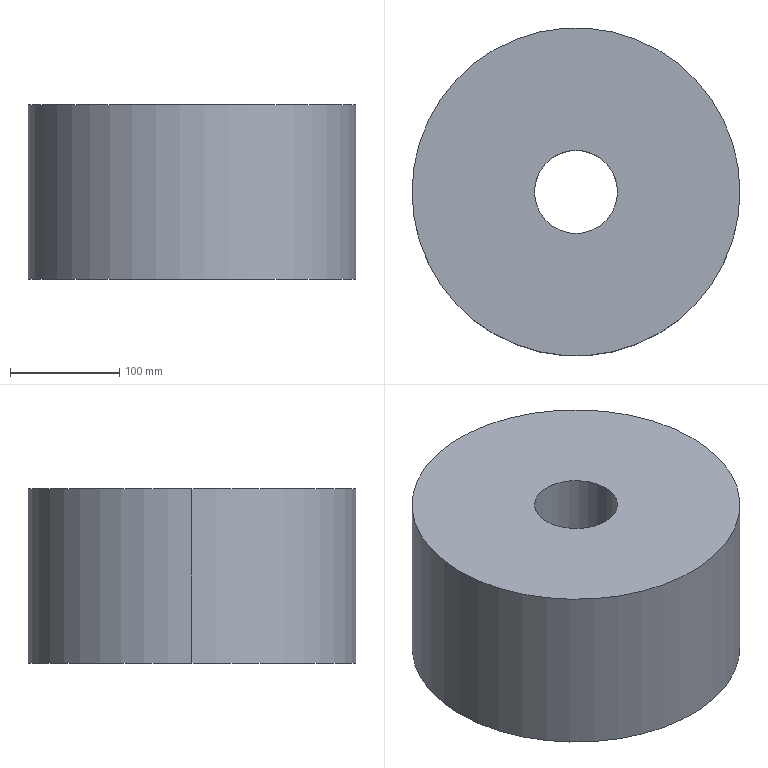Part | SolidWorks | features Extrusion 1 | 1 solid | 6 faces | box 300 x 300 x 160 mm | volume 10583900 mm3 | cylinder 4 | plane 2 | commonest cylinder face diameters 76 x2 300 x2
STEP:
#1=CARTESIAN_POINT('',(-38.,0.,80.));
#2=VERTEX_POINT('',#1);
#3=CARTESIAN_POINT('',(38.,0.,80.));
#4=VERTEX_POINT('',#3);
#5=CARTESIAN_POINT('',(0.,0.,80.));
#6=DIRECTION('',(0.,0.,1.));
#7=DIRECTION('',(1.,0.,0.));
#8=AXIS2_PLACEMENT_3D('',#5,#6,#7);
#9=CIRCLE('',#8,38.);
#10=EDGE_CURVE('',#2,#4,#9,.T.);
#11=ORIENTED_EDGE('',*,*,#10,.T.);
#12=CARTESIAN_POINT('',(38.,0.,-80.));
#13=VERTEX_POINT('',#12);
#14=CARTESIAN_POINT('',(38.,0.,80.));
#15=DIRECTION('',(0.,0.,-1.));
#16=VECTOR('',#15,1000.);
#17=LINE('',#14,#16);
#18=EDGE_CURVE('',#4,#13,#17,.T.);
#19=ORIENTED_EDGE('',*,*,#18,.T.);
#20=CARTESIAN_POINT('',(-38.,0.,-80.));
#21=VERTEX_POINT('',#20);
#22=CARTESIAN_POINT('',(0.,0.,-80.));
#23=DIRECTION('',(0.,0.,1.));
#24=DIRECTION('',(1.,0.,0.));
#25=AXIS2_PLACEMENT_3D('',#22,#23,#24);
#26=CIRCLE('',#25,38.);
#27=EDGE_CURVE('',#21,#13,#26,.T.);
#28=ORIENTED_EDGE('',*,*,#27,.F.);
#29=CARTESIAN_POINT('',(-38.,0.,80.));
#30=DIRECTION('',(0.,0.,-1.));
#31=VECTOR('',#30,1000.);
#32=LINE('',#29,#31);
#33=EDGE_CURVE('',#2,#21,#32,.T.);
#34=ORIENTED_EDGE('',*,*,#33,.F.);
#35=EDGE_LOOP('',(#11,#19,#28,#34));
#36=FACE_OUTER_BOUND('',#35,.T.);
#37=CARTESIAN_POINT('',(0.,0.,80.));
#38=DIRECTION('',(0.,0.,-1.));
#39=DIRECTION('',(-1.,0.,0.));
#40=AXIS2_PLACEMENT_3D('',#37,#38,#39);
#41=CYLINDRICAL_SURFACE('',#40,38.);
#42=ADVANCED_FACE('',(#36),#41,.F.);
#43=CARTESIAN_POINT('',(150.,0.,80.));
#44=VERTEX_POINT('',#43);
#45=CARTESIAN_POINT('',(-150.,0.,80.));
#46=VERTEX_POINT('',#45);
#47=CARTESIAN_POINT('',(0.,0.,80.));
#48=DIRECTION('',(0.,0.,1.));
#49=DIRECTION('',(1.,0.,0.));
#50=AXIS2_PLACEMENT_3D('',#47,#48,#49);
#51=CIRCLE('',#50,150.);
#52=EDGE_CURVE('',#44,#46,#51,.T.);
#53=ORIENTED_EDGE('',*,*,#52,.F.);
#54=CARTESIAN_POINT('',(150.,0.,-80.));
#55=VERTEX_POINT('',#54);
#56=CARTESIAN_POINT('',(150.,0.,80.));
#57=DIRECTION('',(0.,0.,-1.));
#58=VECTOR('',#57,1000.);
#59=LINE('',#56,#58);
#60=EDGE_CURVE('',#44,#55,#59,.T.);
#61=ORIENTED_EDGE('',*,*,#60,.T.);
#62=CARTESIAN_POINT('',(-150.,0.,-80.));
#63=VERTEX_POINT('',#62);
#64=CARTESIAN_POINT('',(0.,0.,-80.));
#65=DIRECTION('',(0.,0.,1.));
#66=DIRECTION('',(1.,0.,0.));
#67=AXIS2_PLACEMENT_3D('',#64,#65,#66);
#68=CIRCLE('',#67,150.);
#69=EDGE_CURVE('',#55,#63,#68,.T.);
#70=ORIENTED_EDGE('',*,*,#69,.T.);
#71=CARTESIAN_POINT('',(-150.,0.,80.));
#72=DIRECTION('',(0.,0.,-1.));
#73=VECTOR('',#72,1000.);
#74=LINE('',#71,#73);
#75=EDGE_CURVE('',#46,#63,#74,.T.);
#76=ORIENTED_EDGE('',*,*,#75,.F.);
#77=EDGE_LOOP('',(#53,#61,#70,#76));
#78=FACE_OUTER_BOUND('',#77,.T.);
#79=CARTESIAN_POINT('',(0.,0.,80.));
#80=DIRECTION('',(0.,0.,-1.));
#81=DIRECTION('',(-1.,0.,0.));
#82=AXIS2_PLACEMENT_3D('',#79,#80,#81);
#83=CYLINDRICAL_SURFACE('',#82,150.);
#84=ADVANCED_FACE('',(#78),#83,.T.);
#85=CARTESIAN_POINT('',(0.,0.,80.));
#86=DIRECTION('',(0.,0.,1.));
#87=DIRECTION('',(1.,0.,0.));
#88=AXIS2_PLACEMENT_3D('',#85,#86,#87);
#89=CIRCLE('',#88,150.);
#90=EDGE_CURVE('',#46,#44,#89,.T.);
#91=ORIENTED_EDGE('',*,*,#90,.T.);
#92=ORIENTED_EDGE('',*,*,#52,.T.);
#93=EDGE_LOOP('',(#91,#92));
#94=FACE_OUTER_BOUND('',#93,.T.);
#95=ORIENTED_EDGE('',*,*,#10,.F.);
#96=CARTESIAN_POINT('',(0.,0.,80.));
#97=DIRECTION('',(0.,0.,1.));
#98=DIRECTION('',(1.,0.,0.));
#99=AXIS2_PLACEMENT_3D('',#96,#97,#98);
#100=CIRCLE('',#99,38.);
#101=EDGE_CURVE('',#4,#2,#100,.T.);
#102=ORIENTED_EDGE('',*,*,#101,.F.);
#103=EDGE_LOOP('',(#95,#102));
#104=FACE_BOUND('',#103,.T.);
#105=CARTESIAN_POINT('',(0.,0.,80.));
#106=DIRECTION('',(0.,0.,1.));
#107=DIRECTION('',(1.,0.,0.));
#108=AXIS2_PLACEMENT_3D('',#105,#106,#107);
#109=PLANE('',#108);
#110=ADVANCED_FACE('',(#94,#104),#109,.T.);
#111=CARTESIAN_POINT('',(0.,0.,-80.));
#112=DIRECTION('',(0.,0.,1.));
#113=DIRECTION('',(1.,0.,0.));
#114=AXIS2_PLACEMENT_3D('',#111,#112,#113);
#115=CIRCLE('',#114,150.);
#116=EDGE_CURVE('',#63,#55,#115,.T.);
#117=ORIENTED_EDGE('',*,*,#116,.F.);
#118=ORIENTED_EDGE('',*,*,#69,.F.);
#119=EDGE_LOOP('',(#117,#118));
#120=FACE_OUTER_BOUND('',#119,.T.);
#121=ORIENTED_EDGE('',*,*,#27,.T.);
#122=CARTESIAN_POINT('',(0.,0.,-80.));
#123=DIRECTION('',(0.,0.,1.));
#124=DIRECTION('',(1.,0.,0.));
#125=AXIS2_PLACEMENT_3D('',#122,#123,#124);
#126=CIRCLE('',#125,38.);
#127=EDGE_CURVE('',#13,#21,#126,.T.);
#128=ORIENTED_EDGE('',*,*,#127,.T.);
#129=EDGE_LOOP('',(#121,#128));
#130=FACE_BOUND('',#129,.T.);
#131=CARTESIAN_POINT('',(0.,0.,-80.));
#132=DIRECTION('',(0.,0.,1.));
#133=DIRECTION('',(1.,0.,0.));
#134=AXIS2_PLACEMENT_3D('',#131,#132,#133);
#135=PLANE('',#134);
#136=ADVANCED_FACE('',(#120,#130),#135,.F.);
#137=ORIENTED_EDGE('',*,*,#60,.F.);
#138=ORIENTED_EDGE('',*,*,#90,.F.);
#139=ORIENTED_EDGE('',*,*,#75,.T.);
#140=ORIENTED_EDGE('',*,*,#116,.T.);
#141=EDGE_LOOP('',(#137,#138,#139,#140));
#142=FACE_OUTER_BOUND('',#141,.T.);
#143=CARTESIAN_POINT('',(0.,0.,80.));
#144=DIRECTION('',(0.,0.,-1.));
#145=DIRECTION('',(-1.,0.,0.));
#146=AXIS2_PLACEMENT_3D('',#143,#144,#145);
#147=CYLINDRICAL_SURFACE('',#146,150.);
#148=ADVANCED_FACE('',(#142),#147,.T.);
#149=ORIENTED_EDGE('',*,*,#18,.F.);
#150=ORIENTED_EDGE('',*,*,#101,.T.);
#151=ORIENTED_EDGE('',*,*,#33,.T.);
#152=ORIENTED_EDGE('',*,*,#127,.F.);
#153=EDGE_LOOP('',(#149,#150,#151,#152));
#154=FACE_OUTER_BOUND('',#153,.T.);
#155=CARTESIAN_POINT('',(0.,0.,80.));
#156=DIRECTION('',(0.,0.,-1.));
#157=DIRECTION('',(-1.,0.,0.));
#158=AXIS2_PLACEMENT_3D('',#155,#156,#157);
#159=CYLINDRICAL_SURFACE('',#158,38.);
#160=ADVANCED_FACE('',(#154),#159,.F.);
#161=CLOSED_SHELL('',(#42,#84,#110,#136,#148,#160));
#162=MANIFOLD_SOLID_BREP('',#161);
#163=CARTESIAN_POINT('',(0.,0.,0.));
#164=DIRECTION('',(0.,0.,1.));
#165=DIRECTION('',(1.,0.,0.));
#166=AXIS2_PLACEMENT_3D('',#163,#164,#165);
#167=(LENGTH_UNIT()NAMED_UNIT(*)SI_UNIT(.MILLI.,.METRE.));
#168=UNCERTAINTY_MEASURE_WITH_UNIT(LENGTH_MEASURE(0.00001),#167,'','');
#169=(NAMED_UNIT(*)PLANE_ANGLE_UNIT()SI_UNIT($,.RADIAN.));
#170=(NAMED_UNIT(*)SI_UNIT($,.STERADIAN.)SOLID_ANGLE_UNIT());
#171=(GEOMETRIC_REPRESENTATION_CONTEXT(3)GLOBAL_UNCERTAINTY_ASSIGNED_CONTEXT((#168))GLOBAL_UNIT_ASSIGNED_CONTEXT((#167,#169,#170))REPRESENTATION_CONTEXT('',''));
#172=ADVANCED_BREP_SHAPE_REPRESENTATION('',(#162,#166),#171);